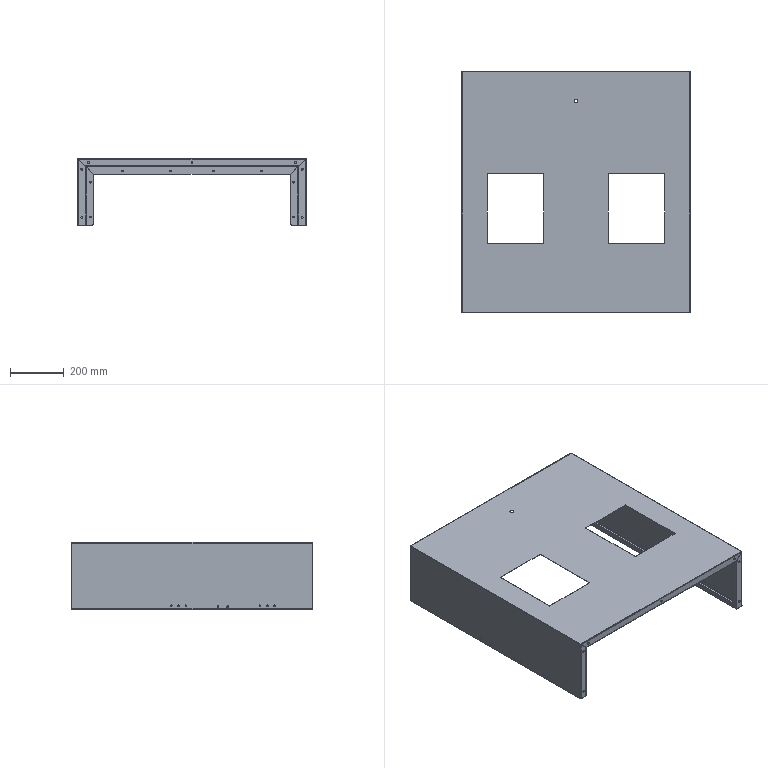Part | SolidWorks | features EdgeFlange 8, ICE 5, HoleWzd 4, Fillet 1, FlatPattern 1, LPattern 1, SMBaseFlange 1, SheetMetal 1 | 1 solid | 312 faces | box 850 x 900 x 250 mm | volume 1614034 mm3 | plane 160 | cylinder 132 | spline 20 | commonest cylinder face diameters 7 x30 6.2 x24 2 x21 4.4 x21 10 x18 6.6 x16